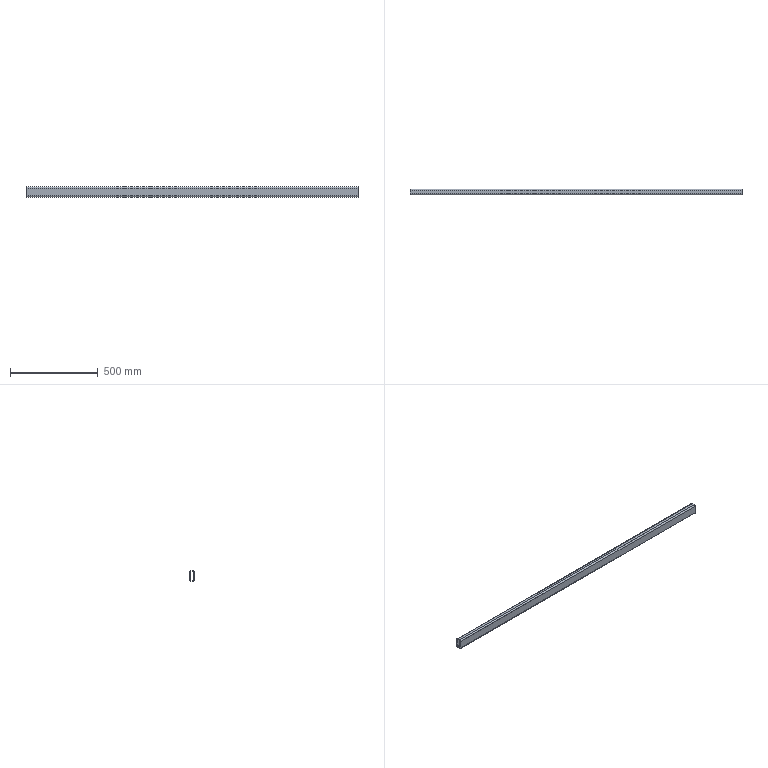Part | STEP file | 1 solid | 18 faces | box 1888 x 30 x 60 mm | volume 1160736 mm3 | plane 10 | cylinder 8 | commonest cylinder face diameters 8 x4 16 x4
STEP:
#1=CARTESIAN_POINT('',(0.,0.,0.));
#2=DIRECTION('',(0.,0.,1.));
#3=DIRECTION('',(1.,0.,0.));
#4=AXIS2_PLACEMENT_3D('',#1,#2,#3);
#5=CARTESIAN_POINT('',(0.,15.,22.));
#6=VERTEX_POINT('',#5);
#7=CARTESIAN_POINT('',(0.,7.,30.));
#8=VERTEX_POINT('',#7);
#9=CARTESIAN_POINT('',(0.,7.,22.));
#10=DIRECTION('',(1.,0.,0.));
#11=DIRECTION('',(0.,0.,-1.));
#12=AXIS2_PLACEMENT_3D('',#9,#10,#11);
#13=CIRCLE('',#12,8.);
#14=CARTESIAN_POINT('',(1888.,7.,22.));
#15=DIRECTION('',(-1.,0.,0.));
#16=DIRECTION('',(0.,0.,1.));
#17=AXIS2_PLACEMENT_3D('',#14,#15,#16);
#18=CYLINDRICAL_SURFACE('',#17,8.);
#19=CARTESIAN_POINT('',(3.142,1888.));
#20=DIRECTION('',(-1.,0.));
#21=VECTOR('',#20,1.);
#22=LINE('',#19,#21);
#23=(GEOMETRIC_REPRESENTATION_CONTEXT(2)PARAMETRIC_REPRESENTATION_CONTEXT()REPRESENTATION_CONTEXT('',''));
#24=DEFINITIONAL_REPRESENTATION('',(#22),#23);
#25=PCURVE('',#18,#24);
#26=CARTESIAN_POINT('',(0.,7.,22.));
#27=DIRECTION('',(1.,0.,0.));
#28=DIRECTION('',(0.,0.,-1.));
#29=AXIS2_PLACEMENT_3D('',#26,#27,#28);
#30=PLANE('',#29);
#31=CARTESIAN_POINT('',(0.,0.));
#32=DIRECTION('',(1.,0.));
#33=AXIS2_PLACEMENT_2D('',#31,#32);
#34=CIRCLE('',#33,8.);
#35=(GEOMETRIC_REPRESENTATION_CONTEXT(2)PARAMETRIC_REPRESENTATION_CONTEXT()REPRESENTATION_CONTEXT('',''));
#36=DEFINITIONAL_REPRESENTATION('',(#34),#35);
#37=PCURVE('',#30,#36);
#38=SURFACE_CURVE('',#13,(#25,#37),.PCURVE_S1.);
#39=EDGE_CURVE('',#6,#8,#38,.T.);
#40=ORIENTED_EDGE('',*,*,#39,.T.);
#41=CARTESIAN_POINT('',(1888.,7.,30.));
#42=VERTEX_POINT('',#41);
#43=CARTESIAN_POINT('',(1888.,7.,30.));
#44=DIRECTION('',(-1.,0.,0.));
#45=VECTOR('',#44,1.);
#46=LINE('',#43,#45);
#47=CARTESIAN_POINT('',(0.,0.));
#48=DIRECTION('',(0.,1.));
#49=VECTOR('',#48,1.);
#50=LINE('',#47,#49);
#51=(GEOMETRIC_REPRESENTATION_CONTEXT(2)PARAMETRIC_REPRESENTATION_CONTEXT()REPRESENTATION_CONTEXT('',''));
#52=DEFINITIONAL_REPRESENTATION('',(#50),#51);
#53=PCURVE('',#18,#52);
#54=CARTESIAN_POINT('',(1888.,7.,30.));
#55=DIRECTION('',(0.,0.,-1.));
#56=DIRECTION('',(-1.,0.,0.));
#57=AXIS2_PLACEMENT_3D('',#54,#55,#56);
#58=PLANE('',#57);
#59=CARTESIAN_POINT('',(0.,0.));
#60=DIRECTION('',(1.,0.));
#61=VECTOR('',#60,1.);
#62=LINE('',#59,#61);
#63=(GEOMETRIC_REPRESENTATION_CONTEXT(2)PARAMETRIC_REPRESENTATION_CONTEXT()REPRESENTATION_CONTEXT('',''));
#64=DEFINITIONAL_REPRESENTATION('',(#62),#63);
#65=PCURVE('',#58,#64);
#66=SURFACE_CURVE('',#46,(#53,#65),.PCURVE_S1.);
#67=EDGE_CURVE('',#42,#8,#66,.T.);
#68=ORIENTED_EDGE('',*,*,#67,.F.);
#69=CARTESIAN_POINT('',(1888.,15.,22.));
#70=VERTEX_POINT('',#69);
#71=CARTESIAN_POINT('',(1888.,7.,22.));
#72=DIRECTION('',(1.,0.,0.));
#73=DIRECTION('',(0.,0.,-1.));
#74=AXIS2_PLACEMENT_3D('',#71,#72,#73);
#75=CIRCLE('',#74,8.);
#76=CARTESIAN_POINT('',(3.142,0.));
#77=DIRECTION('',(-1.,0.));
#78=VECTOR('',#77,1.);
#79=LINE('',#76,#78);
#80=(GEOMETRIC_REPRESENTATION_CONTEXT(2)PARAMETRIC_REPRESENTATION_CONTEXT()REPRESENTATION_CONTEXT('',''));
#81=DEFINITIONAL_REPRESENTATION('',(#79),#80);
#82=PCURVE('',#18,#81);
#83=CARTESIAN_POINT('',(1888.,7.,22.));
#84=DIRECTION('',(1.,0.,0.));
#85=DIRECTION('',(0.,0.,-1.));
#86=AXIS2_PLACEMENT_3D('',#83,#84,#85);
#87=PLANE('',#86);
#88=CARTESIAN_POINT('',(0.,0.));
#89=DIRECTION('',(1.,0.));
#90=AXIS2_PLACEMENT_2D('',#88,#89);
#91=CIRCLE('',#90,8.);
#92=(GEOMETRIC_REPRESENTATION_CONTEXT(2)PARAMETRIC_REPRESENTATION_CONTEXT()REPRESENTATION_CONTEXT('',''));
#93=DEFINITIONAL_REPRESENTATION('',(#91),#92);
#94=PCURVE('',#87,#93);
#95=SURFACE_CURVE('',#75,(#82,#94),.PCURVE_S1.);
#96=EDGE_CURVE('',#70,#42,#95,.T.);
#97=ORIENTED_EDGE('',*,*,#96,.F.);
#98=CARTESIAN_POINT('',(1888.,15.,22.));
#99=DIRECTION('',(-1.,0.,0.));
#100=VECTOR('',#99,1.);
#101=LINE('',#98,#100);
#102=CARTESIAN_POINT('',(1.571,0.));
#103=DIRECTION('',(0.,1.));
#104=VECTOR('',#103,1.);
#105=LINE('',#102,#104);
#106=(GEOMETRIC_REPRESENTATION_CONTEXT(2)PARAMETRIC_REPRESENTATION_CONTEXT()REPRESENTATION_CONTEXT('',''));
#107=DEFINITIONAL_REPRESENTATION('',(#105),#106);
#108=PCURVE('',#18,#107);
#109=CARTESIAN_POINT('',(1888.,15.,22.));
#110=DIRECTION('',(0.,-1.,0.));
#111=DIRECTION('',(0.,0.,-1.));
#112=AXIS2_PLACEMENT_3D('',#109,#110,#111);
#113=PLANE('',#112);
#114=CARTESIAN_POINT('',(0.,0.));
#115=DIRECTION('',(0.,-1.));
#116=VECTOR('',#115,1.);
#117=LINE('',#114,#116);
#118=(GEOMETRIC_REPRESENTATION_CONTEXT(2)PARAMETRIC_REPRESENTATION_CONTEXT()REPRESENTATION_CONTEXT('',''));
#119=DEFINITIONAL_REPRESENTATION('',(#117),#118);
#120=PCURVE('',#113,#119);
#121=SURFACE_CURVE('',#101,(#108,#120),.PCURVE_S1.);
#122=EDGE_CURVE('',#70,#6,#121,.T.);
#123=ORIENTED_EDGE('',*,*,#122,.T.);
#124=EDGE_LOOP('',(#40,#68,#97,#123));
#125=FACE_BOUND('',#124,.T.);
#126=ADVANCED_FACE('',(#125),#18,.T.);
#127=CARTESIAN_POINT('',(0.,-7.,30.));
#128=VERTEX_POINT('',#127);
#129=CARTESIAN_POINT('',(0.,7.,30.));
#130=DIRECTION('',(0.,-1.,0.));
#131=VECTOR('',#130,1.);
#132=LINE('',#129,#131);
#133=CARTESIAN_POINT('',(1888.,0.));
#134=DIRECTION('',(0.,-1.));
#135=VECTOR('',#134,1.);
#136=LINE('',#133,#135);
#137=(GEOMETRIC_REPRESENTATION_CONTEXT(2)PARAMETRIC_REPRESENTATION_CONTEXT()REPRESENTATION_CONTEXT('',''));
#138=DEFINITIONAL_REPRESENTATION('',(#136),#137);
#139=PCURVE('',#58,#138);
#140=CARTESIAN_POINT('',(-8.,0.));
#141=DIRECTION('',(0.,-1.));
#142=VECTOR('',#141,1.);
#143=LINE('',#140,#142);
#144=(GEOMETRIC_REPRESENTATION_CONTEXT(2)PARAMETRIC_REPRESENTATION_CONTEXT()REPRESENTATION_CONTEXT('',''));
#145=DEFINITIONAL_REPRESENTATION('',(#143),#144);
#146=PCURVE('',#30,#145);
#147=SURFACE_CURVE('',#132,(#139,#146),.PCURVE_S1.);
#148=EDGE_CURVE('',#8,#128,#147,.T.);
#149=ORIENTED_EDGE('',*,*,#148,.T.);
#150=CARTESIAN_POINT('',(1888.,-7.,30.));
#151=VERTEX_POINT('',#150);
#152=CARTESIAN_POINT('',(1888.,-7.,30.));
#153=DIRECTION('',(-1.,0.,0.));
#154=VECTOR('',#153,1.);
#155=LINE('',#152,#154);
#156=CARTESIAN_POINT('',(0.,-14.));
#157=DIRECTION('',(1.,0.));
#158=VECTOR('',#157,1.);
#159=LINE('',#156,#158);
#160=(GEOMETRIC_REPRESENTATION_CONTEXT(2)PARAMETRIC_REPRESENTATION_CONTEXT()REPRESENTATION_CONTEXT('',''));
#161=DEFINITIONAL_REPRESENTATION('',(#159),#160);
#162=PCURVE('',#58,#161);
#163=CARTESIAN_POINT('',(1888.,-7.,22.));
#164=DIRECTION('',(-1.,0.,0.));
#165=DIRECTION('',(0.,0.,1.));
#166=AXIS2_PLACEMENT_3D('',#163,#164,#165);
#167=CYLINDRICAL_SURFACE('',#166,8.);
#168=CARTESIAN_POINT('',(6.283,0.));
#169=DIRECTION('',(0.,1.));
#170=VECTOR('',#169,1.);
#171=LINE('',#168,#170);
#172=(GEOMETRIC_REPRESENTATION_CONTEXT(2)PARAMETRIC_REPRESENTATION_CONTEXT()REPRESENTATION_CONTEXT('',''));
#173=DEFINITIONAL_REPRESENTATION('',(#171),#172);
#174=PCURVE('',#167,#173);
#175=SURFACE_CURVE('',#155,(#162,#174),.PCURVE_S1.);
#176=EDGE_CURVE('',#151,#128,#175,.T.);
#177=ORIENTED_EDGE('',*,*,#176,.F.);
#178=CARTESIAN_POINT('',(1888.,7.,30.));
#179=DIRECTION('',(0.,-1.,0.));
#180=VECTOR('',#179,1.);
#181=LINE('',#178,#180);
#182=CARTESIAN_POINT('',(0.,0.));
#183=DIRECTION('',(0.,-1.));
#184=VECTOR('',#183,1.);
#185=LINE('',#182,#184);
#186=(GEOMETRIC_REPRESENTATION_CONTEXT(2)PARAMETRIC_REPRESENTATION_CONTEXT()REPRESENTATION_CONTEXT('',''));
#187=DEFINITIONAL_REPRESENTATION('',(#185),#186);
#188=PCURVE('',#58,#187);
#189=CARTESIAN_POINT('',(-8.,0.));
#190=DIRECTION('',(0.,-1.));
#191=VECTOR('',#190,1.);
#192=LINE('',#189,#191);
#193=(GEOMETRIC_REPRESENTATION_CONTEXT(2)PARAMETRIC_REPRESENTATION_CONTEXT()REPRESENTATION_CONTEXT('',''));
#194=DEFINITIONAL_REPRESENTATION('',(#192),#193);
#195=PCURVE('',#87,#194);
#196=SURFACE_CURVE('',#181,(#188,#195),.PCURVE_S1.);
#197=EDGE_CURVE('',#42,#151,#196,.T.);
#198=ORIENTED_EDGE('',*,*,#197,.F.);
#199=ORIENTED_EDGE('',*,*,#67,.T.);
#200=EDGE_LOOP('',(#149,#177,#198,#199));
#201=FACE_BOUND('',#200,.T.);
#202=ADVANCED_FACE('',(#201),#58,.F.);
#203=CARTESIAN_POINT('',(0.,-15.,22.));
#204=VERTEX_POINT('',#203);
#205=CARTESIAN_POINT('',(0.,-7.,22.));
#206=DIRECTION('',(1.,0.,0.));
#207=DIRECTION('',(0.,0.,-1.));
#208=AXIS2_PLACEMENT_3D('',#205,#206,#207);
#209=CIRCLE('',#208,8.);
#210=CARTESIAN_POINT('',(9.425,1888.));
#211=DIRECTION('',(-1.,0.));
#212=VECTOR('',#211,1.);
#213=LINE('',#210,#212);
#214=(GEOMETRIC_REPRESENTATION_CONTEXT(2)PARAMETRIC_REPRESENTATION_CONTEXT()REPRESENTATION_CONTEXT('',''));
#215=DEFINITIONAL_REPRESENTATION('',(#213),#214);
#216=PCURVE('',#167,#215);
#217=CARTESIAN_POINT('',(0.,-14.));
#218=DIRECTION('',(1.,0.));
#219=AXIS2_PLACEMENT_2D('',#217,#218);
#220=CIRCLE('',#219,8.);
#221=(GEOMETRIC_REPRESENTATION_CONTEXT(2)PARAMETRIC_REPRESENTATION_CONTEXT()REPRESENTATION_CONTEXT('',''));
#222=DEFINITIONAL_REPRESENTATION('',(#220),#221);
#223=PCURVE('',#30,#222);
#224=SURFACE_CURVE('',#209,(#216,#223),.PCURVE_S1.);
#225=EDGE_CURVE('',#128,#204,#224,.T.);
#226=ORIENTED_EDGE('',*,*,#225,.T.);
#227=CARTESIAN_POINT('',(1888.,-15.,22.));
#228=VERTEX_POINT('',#227);
#229=CARTESIAN_POINT('',(1888.,-15.,22.));
#230=DIRECTION('',(-1.,0.,0.));
#231=VECTOR('',#230,1.);
#232=LINE('',#229,#231);
#233=CARTESIAN_POINT('',(4.712,0.));
#234=DIRECTION('',(0.,1.));
#235=VECTOR('',#234,1.);
#236=LINE('',#233,#235);
#237=(GEOMETRIC_REPRESENTATION_CONTEXT(2)PARAMETRIC_REPRESENTATION_CONTEXT()REPRESENTATION_CONTEXT('',''));
#238=DEFINITIONAL_REPRESENTATION('',(#236),#237);
#239=PCURVE('',#167,#238);
#240=CARTESIAN_POINT('',(1888.,-15.,-22.));
#241=DIRECTION('',(0.,1.,0.));
#242=DIRECTION('',(0.,0.,1.));
#243=AXIS2_PLACEMENT_3D('',#240,#241,#242);
#244=PLANE('',#243);
#245=CARTESIAN_POINT('',(44.,0.));
#246=DIRECTION('',(0.,-1.));
#247=VECTOR('',#246,1.);
#248=LINE('',#245,#247);
#249=(GEOMETRIC_REPRESENTATION_CONTEXT(2)PARAMETRIC_REPRESENTATION_CONTEXT()REPRESENTATION_CONTEXT('',''));
#250=DEFINITIONAL_REPRESENTATION('',(#248),#249);
#251=PCURVE('',#244,#250);
#252=SURFACE_CURVE('',#232,(#239,#251),.PCURVE_S1.);
#253=EDGE_CURVE('',#228,#204,#252,.T.);
#254=ORIENTED_EDGE('',*,*,#253,.F.);
#255=CARTESIAN_POINT('',(1888.,-7.,22.));
#256=DIRECTION('',(1.,0.,0.));
#257=DIRECTION('',(0.,0.,-1.));
#258=AXIS2_PLACEMENT_3D('',#255,#256,#257);
#259=CIRCLE('',#258,8.);
#260=CARTESIAN_POINT('',(9.425,0.));
#261=DIRECTION('',(-1.,0.));
#262=VECTOR('',#261,1.);
#263=LINE('',#260,#262);
#264=(GEOMETRIC_REPRESENTATION_CONTEXT(2)PARAMETRIC_REPRESENTATION_CONTEXT()REPRESENTATION_CONTEXT('',''));
#265=DEFINITIONAL_REPRESENTATION('',(#263),#264);
#266=PCURVE('',#167,#265);
#267=CARTESIAN_POINT('',(0.,-14.));
#268=DIRECTION('',(1.,0.));
#269=AXIS2_PLACEMENT_2D('',#267,#268);
#270=CIRCLE('',#269,8.);
#271=(GEOMETRIC_REPRESENTATION_CONTEXT(2)PARAMETRIC_REPRESENTATION_CONTEXT()REPRESENTATION_CONTEXT('',''));
#272=DEFINITIONAL_REPRESENTATION('',(#270),#271);
#273=PCURVE('',#87,#272);
#274=SURFACE_CURVE('',#259,(#266,#273),.PCURVE_S1.);
#275=EDGE_CURVE('',#151,#228,#274,.T.);
#276=ORIENTED_EDGE('',*,*,#275,.F.);
#277=ORIENTED_EDGE('',*,*,#176,.T.);
#278=EDGE_LOOP('',(#226,#254,#276,#277));
#279=FACE_BOUND('',#278,.T.);
#280=ADVANCED_FACE('',(#279),#167,.T.);
#281=CARTESIAN_POINT('',(0.,-15.,-22.));
#282=VERTEX_POINT('',#281);
#283=CARTESIAN_POINT('',(0.,-15.,-22.));
#284=DIRECTION('',(0.,0.,-1.));
#285=VECTOR('',#284,1.);
#286=LINE('',#283,#285);
#287=CARTESIAN_POINT('',(0.,-1888.));
#288=DIRECTION('',(-1.,0.));
#289=VECTOR('',#288,1.);
#290=LINE('',#287,#289);
#291=(GEOMETRIC_REPRESENTATION_CONTEXT(2)PARAMETRIC_REPRESENTATION_CONTEXT()REPRESENTATION_CONTEXT('',''));
#292=DEFINITIONAL_REPRESENTATION('',(#290),#291);
#293=PCURVE('',#244,#292);
#294=CARTESIAN_POINT('',(44.,-22.));
#295=DIRECTION('',(1.,0.));
#296=VECTOR('',#295,1.);
#297=LINE('',#294,#296);
#298=(GEOMETRIC_REPRESENTATION_CONTEXT(2)PARAMETRIC_REPRESENTATION_CONTEXT()REPRESENTATION_CONTEXT('',''));
#299=DEFINITIONAL_REPRESENTATION('',(#297),#298);
#300=PCURVE('',#30,#299);
#301=SURFACE_CURVE('',#286,(#293,#300),.PCURVE_S1.);
#302=EDGE_CURVE('',#204,#282,#301,.T.);
#303=ORIENTED_EDGE('',*,*,#302,.T.);
#304=CARTESIAN_POINT('',(1888.,-15.,-22.));
#305=VERTEX_POINT('',#304);
#306=CARTESIAN_POINT('',(1888.,-15.,-22.));
#307=DIRECTION('',(-1.,0.,0.));
#308=VECTOR('',#307,1.);
#309=LINE('',#306,#308);
#310=CARTESIAN_POINT('',(0.,0.));
#311=DIRECTION('',(0.,-1.));
#312=VECTOR('',#311,1.);
#313=LINE('',#310,#312);
#314=(GEOMETRIC_REPRESENTATION_CONTEXT(2)PARAMETRIC_REPRESENTATION_CONTEXT()REPRESENTATION_CONTEXT('',''));
#315=DEFINITIONAL_REPRESENTATION('',(#313),#314);
#316=PCURVE('',#244,#315);
#317=CARTESIAN_POINT('',(1888.,-7.,-22.));
#318=DIRECTION('',(-1.,0.,0.));
#319=DIRECTION('',(0.,0.,1.));
#320=AXIS2_PLACEMENT_3D('',#317,#318,#319);
#321=CYLINDRICAL_SURFACE('',#320,8.);
#322=CARTESIAN_POINT('',(4.712,0.));
#323=DIRECTION('',(0.,1.));
#324=VECTOR('',#323,1.);
#325=LINE('',#322,#324);
#326=(GEOMETRIC_REPRESENTATION_CONTEXT(2)PARAMETRIC_REPRESENTATION_CONTEXT()REPRESENTATION_CONTEXT('',''));
#327=DEFINITIONAL_REPRESENTATION('',(#325),#326);
#328=PCURVE('',#321,#327);
#329=SURFACE_CURVE('',#309,(#316,#328),.PCURVE_S1.);
#330=EDGE_CURVE('',#305,#282,#329,.T.);
#331=ORIENTED_EDGE('',*,*,#330,.F.);
#332=CARTESIAN_POINT('',(1888.,-15.,-22.));
#333=DIRECTION('',(0.,0.,-1.));
#334=VECTOR('',#333,1.);
#335=LINE('',#332,#334);
#336=CARTESIAN_POINT('',(0.,0.));
#337=DIRECTION('',(-1.,0.));
#338=VECTOR('',#337,1.);
#339=LINE('',#336,#338);
#340=(GEOMETRIC_REPRESENTATION_CONTEXT(2)PARAMETRIC_REPRESENTATION_CONTEXT()REPRESENTATION_CONTEXT('',''));
#341=DEFINITIONAL_REPRESENTATION('',(#339),#340);
#342=PCURVE('',#244,#341);
#343=CARTESIAN_POINT('',(44.,-22.));
#344=DIRECTION('',(1.,0.));
#345=VECTOR('',#344,1.);
#346=LINE('',#343,#345);
#347=(GEOMETRIC_REPRESENTATION_CONTEXT(2)PARAMETRIC_REPRESENTATION_CONTEXT()REPRESENTATION_CONTEXT('',''));
#348=DEFINITIONAL_REPRESENTATION('',(#346),#347);
#349=PCURVE('',#87,#348);
#350=SURFACE_CURVE('',#335,(#342,#349),.PCURVE_S1.);
#351=EDGE_CURVE('',#228,#305,#350,.T.);
#352=ORIENTED_EDGE('',*,*,#351,.F.);
#353=ORIENTED_EDGE('',*,*,#253,.T.);
#354=EDGE_LOOP('',(#303,#331,#352,#353));
#355=FACE_BOUND('',#354,.T.);
#356=ADVANCED_FACE('',(#355),#244,.F.);
#357=CARTESIAN_POINT('',(0.,-7.,-30.));
#358=VERTEX_POINT('',#357);
#359=CARTESIAN_POINT('',(0.,-7.,-22.));
#360=DIRECTION('',(1.,0.,0.));
#361=DIRECTION('',(0.,0.,-1.));
#362=AXIS2_PLACEMENT_3D('',#359,#360,#361);
#363=CIRCLE('',#362,8.);
#364=CARTESIAN_POINT('',(9.425,1888.));
#365=DIRECTION('',(-1.,0.));
#366=VECTOR('',#365,1.);
#367=LINE('',#364,#366);
#368=(GEOMETRIC_REPRESENTATION_CONTEXT(2)PARAMETRIC_REPRESENTATION_CONTEXT()REPRESENTATION_CONTEXT('',''));
#369=DEFINITIONAL_REPRESENTATION('',(#367),#368);
#370=PCURVE('',#321,#369);
#371=CARTESIAN_POINT('',(44.,-14.));
#372=DIRECTION('',(1.,0.));
#373=AXIS2_PLACEMENT_2D('',#371,#372);
#374=CIRCLE('',#373,8.);
#375=(GEOMETRIC_REPRESENTATION_CONTEXT(2)PARAMETRIC_REPRESENTATION_CONTEXT()REPRESENTATION_CONTEXT('',''));
#376=DEFINITIONAL_REPRESENTATION('',(#374),#375);
#377=PCURVE('',#30,#376);
#378=SURFACE_CURVE('',#363,(#370,#377),.PCURVE_S1.);
#379=EDGE_CURVE('',#282,#358,#378,.T.);
#380=ORIENTED_EDGE('',*,*,#379,.T.);
#381=CARTESIAN_POINT('',(1888.,-7.,-30.));
#382=VERTEX_POINT('',#381);
#383=CARTESIAN_POINT('',(1888.,-7.,-30.));
#384=DIRECTION('',(-1.,0.,0.));
#385=VECTOR('',#384,1.);
#386=LINE('',#383,#385);
#387=CARTESIAN_POINT('',(3.142,0.));
#388=DIRECTION('',(0.,1.));
#389=VECTOR('',#388,1.);
#390=LINE('',#387,#389);
#391=(GEOMETRIC_REPRESENTATION_CONTEXT(2)PARAMETRIC_REPRESENTATION_CONTEXT()REPRESENTATION_CONTEXT('',''));
#392=DEFINITIONAL_REPRESENTATION('',(#390),#391);
#393=PCURVE('',#321,#392);
#394=CARTESIAN_POINT('',(1888.,-7.,-30.));
#395=DIRECTION('',(0.,0.,1.));
#396=DIRECTION('',(1.,0.,0.));
#397=AXIS2_PLACEMENT_3D('',#394,#395,#396);
#398=PLANE('',#397);
#399=CARTESIAN_POINT('',(0.,0.));
#400=DIRECTION('',(-1.,0.));
#401=VECTOR('',#400,1.);
#402=LINE('',#399,#401);
#403=(GEOMETRIC_REPRESENTATION_CONTEXT(2)PARAMETRIC_REPRESENTATION_CONTEXT()REPRESENTATION_CONTEXT('',''));
#404=DEFINITIONAL_REPRESENTATION('',(#402),#403);
#405=PCURVE('',#398,#404);
#406=SURFACE_CURVE('',#386,(#393,#405),.PCURVE_S1.);
#407=EDGE_CURVE('',#382,#358,#406,.T.);
#408=ORIENTED_EDGE('',*,*,#407,.F.);
#409=CARTESIAN_POINT('',(1888.,-7.,-22.));
#410=DIRECTION('',(1.,0.,0.));
#411=DIRECTION('',(0.,0.,-1.));
#412=AXIS2_PLACEMENT_3D('',#409,#410,#411);
#413=CIRCLE('',#412,8.);
#414=CARTESIAN_POINT('',(9.425,0.));
#415=DIRECTION('',(-1.,0.));
#416=VECTOR('',#415,1.);
#417=LINE('',#414,#416);
#418=(GEOMETRIC_REPRESENTATION_CONTEXT(2)PARAMETRIC_REPRESENTATION_CONTEXT()REPRESENTATION_CONTEXT('',''));
#419=DEFINITIONAL_REPRESENTATION('',(#417),#418);
#420=PCURVE('',#321,#419);
#421=CARTESIAN_POINT('',(44.,-14.));
#422=DIRECTION('',(1.,0.));
#423=AXIS2_PLACEMENT_2D('',#421,#422);
#424=CIRCLE('',#423,8.);
#425=(GEOMETRIC_REPRESENTATION_CONTEXT(2)PARAMETRIC_REPRESENTATION_CONTEXT()REPRESENTATION_CONTEXT('',''));
#426=DEFINITIONAL_REPRESENTATION('',(#424),#425);
#427=PCURVE('',#87,#426);
#428=SURFACE_CURVE('',#413,(#420,#427),.PCURVE_S1.);
#429=EDGE_CURVE('',#305,#382,#428,.T.);
#430=ORIENTED_EDGE('',*,*,#429,.F.);
#431=ORIENTED_EDGE('',*,*,#330,.T.);
#432=EDGE_LOOP('',(#380,#408,#430,#431));
#433=FACE_BOUND('',#432,.T.);
#434=ADVANCED_FACE('',(#433),#321,.T.);
#435=CARTESIAN_POINT('',(0.,7.,-30.));
#436=VERTEX_POINT('',#435);
#437=CARTESIAN_POINT('',(0.,-7.,-30.));
#438=DIRECTION('',(0.,1.,0.));
#439=VECTOR('',#438,1.);
#440=LINE('',#437,#439);
#441=CARTESIAN_POINT('',(-1888.,0.));
#442=DIRECTION('',(0.,1.));
#443=VECTOR('',#442,1.);
#444=LINE('',#441,#443);
#445=(GEOMETRIC_REPRESENTATION_CONTEXT(2)PARAMETRIC_REPRESENTATION_CONTEXT()REPRESENTATION_CONTEXT('',''));
#446=DEFINITIONAL_REPRESENTATION('',(#444),#445);
#447=PCURVE('',#398,#446);
#448=CARTESIAN_POINT('',(52.,-14.));
#449=DIRECTION('',(0.,1.));
#450=VECTOR('',#449,1.);
#451=LINE('',#448,#450);
#452=(GEOMETRIC_REPRESENTATION_CONTEXT(2)PARAMETRIC_REPRESENTATION_CONTEXT()REPRESENTATION_CONTEXT('',''));
#453=DEFINITIONAL_REPRESENTATION('',(#451),#452);
#454=PCURVE('',#30,#453);
#455=SURFACE_CURVE('',#440,(#447,#454),.PCURVE_S1.);
#456=EDGE_CURVE('',#358,#436,#455,.T.);
#457=ORIENTED_EDGE('',*,*,#456,.T.);
#458=CARTESIAN_POINT('',(1888.,7.,-30.));
#459=VERTEX_POINT('',#458);
#460=CARTESIAN_POINT('',(1888.,7.,-30.));
#461=DIRECTION('',(-1.,0.,0.));
#462=VECTOR('',#461,1.);
#463=LINE('',#460,#462);
#464=CARTESIAN_POINT('',(0.,14.));
#465=DIRECTION('',(-1.,0.));
#466=VECTOR('',#465,1.);
#467=LINE('',#464,#466);
#468=(GEOMETRIC_REPRESENTATION_CONTEXT(2)PARAMETRIC_REPRESENTATION_CONTEXT()REPRESENTATION_CONTEXT('',''));
#469=DEFINITIONAL_REPRESENTATION('',(#467),#468);
#470=PCURVE('',#398,#469);
#471=CARTESIAN_POINT('',(1888.,7.,-22.));
#472=DIRECTION('',(-1.,0.,0.));
#473=DIRECTION('',(0.,0.,1.));
#474=AXIS2_PLACEMENT_3D('',#471,#472,#473);
#475=CYLINDRICAL_SURFACE('',#474,8.);
#476=CARTESIAN_POINT('',(3.142,0.));
#477=DIRECTION('',(0.,1.));
#478=VECTOR('',#477,1.);
#479=LINE('',#476,#478);
#480=(GEOMETRIC_REPRESENTATION_CONTEXT(2)PARAMETRIC_REPRESENTATION_CONTEXT()REPRESENTATION_CONTEXT('',''));
#481=DEFINITIONAL_REPRESENTATION('',(#479),#480);
#482=PCURVE('',#475,#481);
#483=SURFACE_CURVE('',#463,(#470,#482),.PCURVE_S1.);
#484=EDGE_CURVE('',#459,#436,#483,.T.);
#485=ORIENTED_EDGE('',*,*,#484,.F.);
#486=CARTESIAN_POINT('',(1888.,-7.,-30.));
#487=DIRECTION('',(0.,1.,0.));
#488=VECTOR('',#487,1.);
#489=LINE('',#486,#488);
#490=CARTESIAN_POINT('',(0.,0.));
#491=DIRECTION('',(0.,1.));
#492=VECTOR('',#491,1.);
#493=LINE('',#490,#492);
#494=(GEOMETRIC_REPRESENTATION_CONTEXT(2)PARAMETRIC_REPRESENTATION_CONTEXT()REPRESENTATION_CONTEXT('',''));
#495=DEFINITIONAL_REPRESENTATION('',(#493),#494);
#496=PCURVE('',#398,#495);
#497=CARTESIAN_POINT('',(52.,-14.));
#498=DIRECTION('',(0.,1.));
#499=VECTOR('',#498,1.);
#500=LINE('',#497,#499);
#501=(GEOMETRIC_REPRESENTATION_CONTEXT(2)PARAMETRIC_REPRESENTATION_CONTEXT()REPRESENTATION_CONTEXT('',''));
#502=DEFINITIONAL_REPRESENTATION('',(#500),#501);
#503=PCURVE('',#87,#502);
#504=SURFACE_CURVE('',#489,(#496,#503),.PCURVE_S1.);
#505=EDGE_CURVE('',#382,#459,#504,.T.);
#506=ORIENTED_EDGE('',*,*,#505,.F.);
#507=ORIENTED_EDGE('',*,*,#407,.T.);
#508=EDGE_LOOP('',(#457,#485,#506,#507));
#509=FACE_BOUND('',#508,.T.);
#510=ADVANCED_FACE('',(#509),#398,.F.);
#511=CARTESIAN_POINT('',(0.,15.,-22.));
#512=VERTEX_POINT('',#511);
#513=CARTESIAN_POINT('',(0.,7.,-22.));
#514=DIRECTION('',(1.,0.,0.));
#515=DIRECTION('',(0.,0.,-1.));
#516=AXIS2_PLACEMENT_3D('',#513,#514,#515);
#517=CIRCLE('',#516,8.);
#518=CARTESIAN_POINT('',(3.142,1888.));
#519=DIRECTION('',(-1.,0.));
#520=VECTOR('',#519,1.);
#521=LINE('',#518,#520);
#522=(GEOMETRIC_REPRESENTATION_CONTEXT(2)PARAMETRIC_REPRESENTATION_CONTEXT()REPRESENTATION_CONTEXT('',''));
#523=DEFINITIONAL_REPRESENTATION('',(#521),#522);
#524=PCURVE('',#475,#523);
#525=CARTESIAN_POINT('',(44.,0.));
#526=DIRECTION('',(1.,0.));
#527=AXIS2_PLACEMENT_2D('',#525,#526);
#528=CIRCLE('',#527,8.);
#529=(GEOMETRIC_REPRESENTATION_CONTEXT(2)PARAMETRIC_REPRESENTATION_CONTEXT()REPRESENTATION_CONTEXT('',''));
#530=DEFINITIONAL_REPRESENTATION('',(#528),#529);
#531=PCURVE('',#30,#530);
#532=SURFACE_CURVE('',#517,(#524,#531),.PCURVE_S1.);
#533=EDGE_CURVE('',#436,#512,#532,.T.);
#534=ORIENTED_EDGE('',*,*,#533,.T.);
#535=CARTESIAN_POINT('',(1888.,15.,-22.));
#536=VERTEX_POINT('',#535);
#537=CARTESIAN_POINT('',(1888.,15.,-22.));
#538=DIRECTION('',(-1.,0.,0.));
#539=VECTOR('',#538,1.);
#540=LINE('',#537,#539);
#541=CARTESIAN_POINT('',(1.571,0.));
#542=DIRECTION('',(0.,1.));
#543=VECTOR('',#542,1.);
#544=LINE('',#541,#543);
#545=(GEOMETRIC_REPRESENTATION_CONTEXT(2)PARAMETRIC_REPRESENTATION_CONTEXT()REPRESENTATION_CONTEXT('',''));
#546=DEFINITIONAL_REPRESENTATION('',(#544),#545);
#547=PCURVE('',#475,#546);
#548=CARTESIAN_POINT('',(44.,0.));
#549=DIRECTION('',(0.,-1.));
#550=VECTOR('',#549,1.);
#551=LINE('',#548,#550);
#552=(GEOMETRIC_REPRESENTATION_CONTEXT(2)PARAMETRIC_REPRESENTATION_CONTEXT()REPRESENTATION_CONTEXT('',''));
#553=DEFINITIONAL_REPRESENTATION('',(#551),#552);
#554=PCURVE('',#113,#553);
#555=SURFACE_CURVE('',#540,(#547,#554),.PCURVE_S1.);
#556=EDGE_CURVE('',#536,#512,#555,.T.);
#557=ORIENTED_EDGE('',*,*,#556,.F.);
#558=CARTESIAN_POINT('',(1888.,7.,-22.));
#559=DIRECTION('',(1.,0.,0.));
#560=DIRECTION('',(0.,0.,-1.));
#561=AXIS2_PLACEMENT_3D('',#558,#559,#560);
#562=CIRCLE('',#561,8.);
#563=CARTESIAN_POINT('',(3.142,0.));
#564=DIRECTION('',(-1.,0.));
#565=VECTOR('',#564,1.);
#566=LINE('',#563,#565);
#567=(GEOMETRIC_REPRESENTATION_CONTEXT(2)PARAMETRIC_REPRESENTATION_CONTEXT()REPRESENTATION_CONTEXT('',''));
#568=DEFINITIONAL_REPRESENTATION('',(#566),#567);
#569=PCURVE('',#475,#568);
#570=CARTESIAN_POINT('',(44.,0.));
#571=DIRECTION('',(1.,0.));
#572=AXIS2_PLACEMENT_2D('',#570,#571);
#573=CIRCLE('',#572,8.);
#574=(GEOMETRIC_REPRESENTATION_CONTEXT(2)PARAMETRIC_REPRESENTATION_CONTEXT()REPRESENTATION_CONTEXT('',''));
#575=DEFINITIONAL_REPRESENTATION('',(#573),#574);
#576=PCURVE('',#87,#575);
#577=SURFACE_CURVE('',#562,(#569,#576),.PCURVE_S1.);
#578=EDGE_CURVE('',#459,#536,#577,.T.);
#579=ORIENTED_EDGE('',*,*,#578,.F.);
#580=ORIENTED_EDGE('',*,*,#484,.T.);
#581=EDGE_LOOP('',(#534,#557,#579,#580));
#582=FACE_BOUND('',#581,.T.);
#583=ADVANCED_FACE('',(#582),#475,.T.);
#584=CARTESIAN_POINT('',(1888.,-11.,22.));
#585=VERTEX_POINT('',#584);
#586=CARTESIAN_POINT('',(0.,-11.,22.));
#587=VERTEX_POINT('',#586);
#588=CARTESIAN_POINT('',(1888.,-11.,22.));
#589=DIRECTION('',(-1.,0.,0.));
#590=VECTOR('',#589,1.);
#591=LINE('',#588,#590);
#592=CARTESIAN_POINT('',(1888.,-7.,22.));
#593=DIRECTION('',(-1.,0.,0.));
#594=DIRECTION('',(0.,0.,1.));
#595=AXIS2_PLACEMENT_3D('',#592,#593,#594);
#596=CYLINDRICAL_SURFACE('',#595,4.);
#597=CARTESIAN_POINT('',(4.712,0.));
#598=DIRECTION('',(0.,1.));
#599=VECTOR('',#598,1.);
#600=LINE('',#597,#599);
#601=(GEOMETRIC_REPRESENTATION_CONTEXT(2)PARAMETRIC_REPRESENTATION_CONTEXT()REPRESENTATION_CONTEXT('',''));
#602=DEFINITIONAL_REPRESENTATION('',(#600),#601);
#603=PCURVE('',#596,#602);
#604=CARTESIAN_POINT('',(1888.,-11.,-22.));
#605=DIRECTION('',(0.,1.,0.));
#606=DIRECTION('',(0.,0.,1.));
#607=AXIS2_PLACEMENT_3D('',#604,#605,#606);
#608=PLANE('',#607);
#609=CARTESIAN_POINT('',(44.,0.));
#610=DIRECTION('',(0.,-1.));
#611=VECTOR('',#610,1.);
#612=LINE('',#609,#611);
#613=(GEOMETRIC_REPRESENTATION_CONTEXT(2)PARAMETRIC_REPRESENTATION_CONTEXT()REPRESENTATION_CONTEXT('',''));
#614=DEFINITIONAL_REPRESENTATION('',(#612),#613);
#615=PCURVE('',#608,#614);
#616=SURFACE_CURVE('',#591,(#603,#615),.PCURVE_S1.);
#617=EDGE_CURVE('',#585,#587,#616,.T.);
#618=ORIENTED_EDGE('',*,*,#617,.F.);
#619=CARTESIAN_POINT('',(1888.,-7.,26.));
#620=VERTEX_POINT('',#619);
#621=CARTESIAN_POINT('',(1888.,-7.,22.));
#622=DIRECTION('',(1.,0.,0.));
#623=DIRECTION('',(0.,0.,-1.));
#624=AXIS2_PLACEMENT_3D('',#621,#622,#623);
#625=CIRCLE('',#624,4.);
#626=CARTESIAN_POINT('',(9.425,0.));
#627=DIRECTION('',(-1.,0.));
#628=VECTOR('',#627,1.);
#629=LINE('',#626,#628);
#630=(GEOMETRIC_REPRESENTATION_CONTEXT(2)PARAMETRIC_REPRESENTATION_CONTEXT()REPRESENTATION_CONTEXT('',''));
#631=DEFINITIONAL_REPRESENTATION('',(#629),#630);
#632=PCURVE('',#596,#631);
#633=CARTESIAN_POINT('',(0.,-14.));
#634=DIRECTION('',(1.,0.));
#635=AXIS2_PLACEMENT_2D('',#633,#634);
#636=CIRCLE('',#635,4.);
#637=(GEOMETRIC_REPRESENTATION_CONTEXT(2)PARAMETRIC_REPRESENTATION_CONTEXT()REPRESENTATION_CONTEXT('',''));
#638=DEFINITIONAL_REPRESENTATION('',(#636),#637);
#639=PCURVE('',#87,#638);
#640=SURFACE_CURVE('',#625,(#632,#639),.PCURVE_S1.);
#641=EDGE_CURVE('',#620,#585,#640,.T.);
#642=ORIENTED_EDGE('',*,*,#641,.F.);
#643=CARTESIAN_POINT('',(0.,-7.,26.));
#644=VERTEX_POINT('',#643);
#645=CARTESIAN_POINT('',(1888.,-7.,26.));
#646=DIRECTION('',(-1.,0.,0.));
#647=VECTOR('',#646,1.);
#648=LINE('',#645,#647);
#649=CARTESIAN_POINT('',(6.283,0.));
#650=DIRECTION('',(0.,1.));
#651=VECTOR('',#650,1.);
#652=LINE('',#649,#651);
#653=(GEOMETRIC_REPRESENTATION_CONTEXT(2)PARAMETRIC_REPRESENTATION_CONTEXT()REPRESENTATION_CONTEXT('',''));
#654=DEFINITIONAL_REPRESENTATION('',(#652),#653);
#655=PCURVE('',#596,#654);
#656=CARTESIAN_POINT('',(1888.,7.,26.));
#657=DIRECTION('',(0.,0.,-1.));
#658=DIRECTION('',(-1.,0.,0.));
#659=AXIS2_PLACEMENT_3D('',#656,#657,#658);
#660=PLANE('',#659);
#661=CARTESIAN_POINT('',(0.,-14.));
#662=DIRECTION('',(1.,0.));
#663=VECTOR('',#662,1.);
#664=LINE('',#661,#663);
#665=(GEOMETRIC_REPRESENTATION_CONTEXT(2)PARAMETRIC_REPRESENTATION_CONTEXT()REPRESENTATION_CONTEXT('',''));
#666=DEFINITIONAL_REPRESENTATION('',(#664),#665);
#667=PCURVE('',#660,#666);
#668=SURFACE_CURVE('',#648,(#655,#667),.PCURVE_S1.);
#669=EDGE_CURVE('',#620,#644,#668,.T.);
#670=ORIENTED_EDGE('',*,*,#669,.T.);
#671=CARTESIAN_POINT('',(0.,-7.,22.));
#672=DIRECTION('',(1.,0.,0.));
#673=DIRECTION('',(0.,0.,-1.));
#674=AXIS2_PLACEMENT_3D('',#671,#672,#673);
#675=CIRCLE('',#674,4.);
#676=CARTESIAN_POINT('',(9.425,1888.));
#677=DIRECTION('',(-1.,0.));
#678=VECTOR('',#677,1.);
#679=LINE('',#676,#678);
#680=(GEOMETRIC_REPRESENTATION_CONTEXT(2)PARAMETRIC_REPRESENTATION_CONTEXT()REPRESENTATION_CONTEXT('',''));
#681=DEFINITIONAL_REPRESENTATION('',(#679),#680);
#682=PCURVE('',#596,#681);
#683=CARTESIAN_POINT('',(0.,-14.));
#684=DIRECTION('',(1.,0.));
#685=AXIS2_PLACEMENT_2D('',#683,#684);
#686=CIRCLE('',#685,4.);
#687=(GEOMETRIC_REPRESENTATION_CONTEXT(2)PARAMETRIC_REPRESENTATION_CONTEXT()REPRESENTATION_CONTEXT('',''));
#688=DEFINITIONAL_REPRESENTATION('',(#686),#687);
#689=PCURVE('',#30,#688);
#690=SURFACE_CURVE('',#675,(#682,#689),.PCURVE_S1.);
#691=EDGE_CURVE('',#644,#587,#690,.T.);
#692=ORIENTED_EDGE('',*,*,#691,.T.);
#693=EDGE_LOOP('',(#618,#642,#670,#692));
#694=FACE_BOUND('',#693,.F.);
#695=ADVANCED_FACE('',(#694),#596,.F.);
#696=CARTESIAN_POINT('',(0.,7.,26.));
#697=VERTEX_POINT('',#696);
#698=CARTESIAN_POINT('',(0.,7.,26.));
#699=DIRECTION('',(0.,-1.,0.));
#700=VECTOR('',#699,1.);
#701=LINE('',#698,#700);
#702=CARTESIAN_POINT('',(1888.,0.));
#703=DIRECTION('',(0.,-1.));
#704=VECTOR('',#703,1.);
#705=LINE('',#702,#704);
#706=(GEOMETRIC_REPRESENTATION_CONTEXT(2)PARAMETRIC_REPRESENTATION_CONTEXT()REPRESENTATION_CONTEXT('',''));
#707=DEFINITIONAL_REPRESENTATION('',(#705),#706);
#708=PCURVE('',#660,#707);
#709=CARTESIAN_POINT('',(-4.,0.));
#710=DIRECTION('',(0.,-1.));
#711=VECTOR('',#710,1.);
#712=LINE('',#709,#711);
#713=(GEOMETRIC_REPRESENTATION_CONTEXT(2)PARAMETRIC_REPRESENTATION_CONTEXT()REPRESENTATION_CONTEXT('',''));
#714=DEFINITIONAL_REPRESENTATION('',(#712),#713);
#715=PCURVE('',#30,#714);
#716=SURFACE_CURVE('',#701,(#708,#715),.PCURVE_S1.);
#717=EDGE_CURVE('',#697,#644,#716,.T.);
#718=ORIENTED_EDGE('',*,*,#717,.F.);
#719=CARTESIAN_POINT('',(1888.,7.,26.));
#720=VERTEX_POINT('',#719);
#721=CARTESIAN_POINT('',(1888.,7.,26.));
#722=DIRECTION('',(-1.,0.,0.));
#723=VECTOR('',#722,1.);
#724=LINE('',#721,#723);
#725=CARTESIAN_POINT('',(0.,0.));
#726=DIRECTION('',(1.,0.));
#727=VECTOR('',#726,1.);
#728=LINE('',#725,#727);
#729=(GEOMETRIC_REPRESENTATION_CONTEXT(2)PARAMETRIC_REPRESENTATION_CONTEXT()REPRESENTATION_CONTEXT('',''));
#730=DEFINITIONAL_REPRESENTATION('',(#728),#729);
#731=PCURVE('',#660,#730);
#732=CARTESIAN_POINT('',(1888.,7.,22.));
#733=DIRECTION('',(-1.,0.,0.));
#734=DIRECTION('',(0.,0.,1.));
#735=AXIS2_PLACEMENT_3D('',#732,#733,#734);
#736=CYLINDRICAL_SURFACE('',#735,4.);
#737=CARTESIAN_POINT('',(0.,0.));
#738=DIRECTION('',(0.,1.));
#739=VECTOR('',#738,1.);
#740=LINE('',#737,#739);
#741=(GEOMETRIC_REPRESENTATION_CONTEXT(2)PARAMETRIC_REPRESENTATION_CONTEXT()REPRESENTATION_CONTEXT('',''));
#742=DEFINITIONAL_REPRESENTATION('',(#740),#741);
#743=PCURVE('',#736,#742);
#744=SURFACE_CURVE('',#724,(#731,#743),.PCURVE_S1.);
#745=EDGE_CURVE('',#720,#697,#744,.T.);
#746=ORIENTED_EDGE('',*,*,#745,.F.);
#747=CARTESIAN_POINT('',(1888.,7.,26.));
#748=DIRECTION('',(0.,-1.,0.));
#749=VECTOR('',#748,1.);
#750=LINE('',#747,#749);
#751=CARTESIAN_POINT('',(0.,0.));
#752=DIRECTION('',(0.,-1.));
#753=VECTOR('',#752,1.);
#754=LINE('',#751,#753);
#755=(GEOMETRIC_REPRESENTATION_CONTEXT(2)PARAMETRIC_REPRESENTATION_CONTEXT()REPRESENTATION_CONTEXT('',''));
#756=DEFINITIONAL_REPRESENTATION('',(#754),#755);
#757=PCURVE('',#660,#756);
#758=CARTESIAN_POINT('',(-4.,0.));
#759=DIRECTION('',(0.,-1.));
#760=VECTOR('',#759,1.);
#761=LINE('',#758,#760);
#762=(GEOMETRIC_REPRESENTATION_CONTEXT(2)PARAMETRIC_REPRESENTATION_CONTEXT()REPRESENTATION_CONTEXT('',''));
#763=DEFINITIONAL_REPRESENTATION('',(#761),#762);
#764=PCURVE('',#87,#763);
#765=SURFACE_CURVE('',#750,(#757,#764),.PCURVE_S1.);
#766=EDGE_CURVE('',#720,#620,#765,.T.);
#767=ORIENTED_EDGE('',*,*,#766,.T.);
#768=ORIENTED_EDGE('',*,*,#669,.T.);
#769=EDGE_LOOP('',(#718,#746,#767,#768));
#770=FACE_BOUND('',#769,.T.);
#771=ADVANCED_FACE('',(#770),#660,.T.);
#772=ORIENTED_EDGE('',*,*,#745,.F.);
#773=CARTESIAN_POINT('',(1888.,11.,22.));
#774=VERTEX_POINT('',#773);
#775=CARTESIAN_POINT('',(1888.,7.,22.));
#776=DIRECTION('',(1.,0.,0.));
#777=DIRECTION('',(0.,0.,-1.));
#778=AXIS2_PLACEMENT_3D('',#775,#776,#777);
#779=CIRCLE('',#778,4.);
#780=CARTESIAN_POINT('',(3.142,0.));
#781=DIRECTION('',(-1.,0.));
#782=VECTOR('',#781,1.);
#783=LINE('',#780,#782);
#784=(GEOMETRIC_REPRESENTATION_CONTEXT(2)PARAMETRIC_REPRESENTATION_CONTEXT()REPRESENTATION_CONTEXT('',''));
#785=DEFINITIONAL_REPRESENTATION('',(#783),#784);
#786=PCURVE('',#736,#785);
#787=CARTESIAN_POINT('',(0.,0.));
#788=DIRECTION('',(1.,0.));
#789=AXIS2_PLACEMENT_2D('',#787,#788);
#790=CIRCLE('',#789,4.);
#791=(GEOMETRIC_REPRESENTATION_CONTEXT(2)PARAMETRIC_REPRESENTATION_CONTEXT()REPRESENTATION_CONTEXT('',''));
#792=DEFINITIONAL_REPRESENTATION('',(#790),#791);
#793=PCURVE('',#87,#792);
#794=SURFACE_CURVE('',#779,(#786,#793),.PCURVE_S1.);
#795=EDGE_CURVE('',#774,#720,#794,.T.);
#796=ORIENTED_EDGE('',*,*,#795,.F.);
#797=CARTESIAN_POINT('',(0.,11.,22.));
#798=VERTEX_POINT('',#797);
#799=CARTESIAN_POINT('',(1888.,11.,22.));
#800=DIRECTION('',(-1.,0.,0.));
#801=VECTOR('',#800,1.);
#802=LINE('',#799,#801);
#803=CARTESIAN_POINT('',(1.571,0.));
#804=DIRECTION('',(0.,1.));
#805=VECTOR('',#804,1.);
#806=LINE('',#803,#805);
#807=(GEOMETRIC_REPRESENTATION_CONTEXT(2)PARAMETRIC_REPRESENTATION_CONTEXT()REPRESENTATION_CONTEXT('',''));
#808=DEFINITIONAL_REPRESENTATION('',(#806),#807);
#809=PCURVE('',#736,#808);
#810=CARTESIAN_POINT('',(1888.,11.,22.));
#811=DIRECTION('',(0.,-1.,0.));
#812=DIRECTION('',(0.,0.,-1.));
#813=AXIS2_PLACEMENT_3D('',#810,#811,#812);
#814=PLANE('',#813);
#815=CARTESIAN_POINT('',(0.,0.));
#816=DIRECTION('',(0.,-1.));
#817=VECTOR('',#816,1.);
#818=LINE('',#815,#817);
#819=(GEOMETRIC_REPRESENTATION_CONTEXT(2)PARAMETRIC_REPRESENTATION_CONTEXT()REPRESENTATION_CONTEXT('',''));
#820=DEFINITIONAL_REPRESENTATION('',(#818),#819);
#821=PCURVE('',#814,#820);
#822=SURFACE_CURVE('',#802,(#809,#821),.PCURVE_S1.);
#823=EDGE_CURVE('',#774,#798,#822,.T.);
#824=ORIENTED_EDGE('',*,*,#823,.T.);
#825=CARTESIAN_POINT('',(0.,7.,22.));
#826=DIRECTION('',(1.,0.,0.));
#827=DIRECTION('',(0.,0.,-1.));
#828=AXIS2_PLACEMENT_3D('',#825,#826,#827);
#829=CIRCLE('',#828,4.);
#830=CARTESIAN_POINT('',(3.142,1888.));
#831=DIRECTION('',(-1.,0.));
#832=VECTOR('',#831,1.);
#833=LINE('',#830,#832);
#834=(GEOMETRIC_REPRESENTATION_CONTEXT(2)PARAMETRIC_REPRESENTATION_CONTEXT()REPRESENTATION_CONTEXT('',''));
#835=DEFINITIONAL_REPRESENTATION('',(#833),#834);
#836=PCURVE('',#736,#835);
#837=CARTESIAN_POINT('',(0.,0.));
#838=DIRECTION('',(1.,0.));
#839=AXIS2_PLACEMENT_2D('',#837,#838);
#840=CIRCLE('',#839,4.);
#841=(GEOMETRIC_REPRESENTATION_CONTEXT(2)PARAMETRIC_REPRESENTATION_CONTEXT()REPRESENTATION_CONTEXT('',''));
#842=DEFINITIONAL_REPRESENTATION('',(#840),#841);
#843=PCURVE('',#30,#842);
#844=SURFACE_CURVE('',#829,(#836,#843),.PCURVE_S1.);
#845=EDGE_CURVE('',#798,#697,#844,.T.);
#846=ORIENTED_EDGE('',*,*,#845,.T.);
#847=EDGE_LOOP('',(#772,#796,#824,#846));
#848=FACE_BOUND('',#847,.F.);
#849=ADVANCED_FACE('',(#848),#736,.F.);
#850=CARTESIAN_POINT('',(0.,11.,-22.));
#851=VERTEX_POINT('',#850);
#852=CARTESIAN_POINT('',(0.,11.,22.));
#853=DIRECTION('',(0.,0.,1.));
#854=VECTOR('',#853,1.);
#855=LINE('',#852,#854);
#856=CARTESIAN_POINT('',(0.,-1888.));
#857=DIRECTION('',(-1.,0.));
#858=VECTOR('',#857,1.);
#859=LINE('',#856,#858);
#860=(GEOMETRIC_REPRESENTATION_CONTEXT(2)PARAMETRIC_REPRESENTATION_CONTEXT()REPRESENTATION_CONTEXT('',''));
#861=DEFINITIONAL_REPRESENTATION('',(#859),#860);
#862=PCURVE('',#814,#861);
#863=CARTESIAN_POINT('',(0.,4.));
#864=DIRECTION('',(-1.,0.));
#865=VECTOR('',#864,1.);
#866=LINE('',#863,#865);
#867=(GEOMETRIC_REPRESENTATION_CONTEXT(2)PARAMETRIC_REPRESENTATION_CONTEXT()REPRESENTATION_CONTEXT('',''));
#868=DEFINITIONAL_REPRESENTATION('',(#866),#867);
#869=PCURVE('',#30,#868);
#870=SURFACE_CURVE('',#855,(#862,#869),.PCURVE_S1.);
#871=EDGE_CURVE('',#851,#798,#870,.T.);
#872=ORIENTED_EDGE('',*,*,#871,.F.);
#873=CARTESIAN_POINT('',(1888.,11.,-22.));
#874=VERTEX_POINT('',#873);
#875=CARTESIAN_POINT('',(1888.,11.,-22.));
#876=DIRECTION('',(-1.,0.,0.));
#877=VECTOR('',#876,1.);
#878=LINE('',#875,#877);
#879=CARTESIAN_POINT('',(44.,0.));
#880=DIRECTION('',(0.,-1.));
#881=VECTOR('',#880,1.);
#882=LINE('',#879,#881);
#883=(GEOMETRIC_REPRESENTATION_CONTEXT(2)PARAMETRIC_REPRESENTATION_CONTEXT()REPRESENTATION_CONTEXT('',''));
#884=DEFINITIONAL_REPRESENTATION('',(#882),#883);
#885=PCURVE('',#814,#884);
#886=CARTESIAN_POINT('',(1888.,7.,-22.));
#887=DIRECTION('',(-1.,0.,0.));
#888=DIRECTION('',(0.,0.,1.));
#889=AXIS2_PLACEMENT_3D('',#886,#887,#888);
#890=CYLINDRICAL_SURFACE('',#889,4.);
#891=CARTESIAN_POINT('',(1.571,0.));
#892=DIRECTION('',(0.,1.));
#893=VECTOR('',#892,1.);
#894=LINE('',#891,#893);
#895=(GEOMETRIC_REPRESENTATION_CONTEXT(2)PARAMETRIC_REPRESENTATION_CONTEXT()REPRESENTATION_CONTEXT('',''));
#896=DEFINITIONAL_REPRESENTATION('',(#894),#895);
#897=PCURVE('',#890,#896);
#898=SURFACE_CURVE('',#878,(#885,#897),.PCURVE_S1.);
#899=EDGE_CURVE('',#874,#851,#898,.T.);
#900=ORIENTED_EDGE('',*,*,#899,.F.);
#901=CARTESIAN_POINT('',(1888.,11.,22.));
#902=DIRECTION('',(0.,0.,1.));
#903=VECTOR('',#902,1.);
#904=LINE('',#901,#903);
#905=CARTESIAN_POINT('',(0.,0.));
#906=DIRECTION('',(-1.,0.));
#907=VECTOR('',#906,1.);
#908=LINE('',#905,#907);
#909=(GEOMETRIC_REPRESENTATION_CONTEXT(2)PARAMETRIC_REPRESENTATION_CONTEXT()REPRESENTATION_CONTEXT('',''));
#910=DEFINITIONAL_REPRESENTATION('',(#908),#909);
#911=PCURVE('',#814,#910);
#912=CARTESIAN_POINT('',(0.,4.));
#913=DIRECTION('',(-1.,0.));
#914=VECTOR('',#913,1.);
#915=LINE('',#912,#914);
#916=(GEOMETRIC_REPRESENTATION_CONTEXT(2)PARAMETRIC_REPRESENTATION_CONTEXT()REPRESENTATION_CONTEXT('',''));
#917=DEFINITIONAL_REPRESENTATION('',(#915),#916);
#918=PCURVE('',#87,#917);
#919=SURFACE_CURVE('',#904,(#911,#918),.PCURVE_S1.);
#920=EDGE_CURVE('',#874,#774,#919,.T.);
#921=ORIENTED_EDGE('',*,*,#920,.T.);
#922=ORIENTED_EDGE('',*,*,#823,.T.);
#923=EDGE_LOOP('',(#872,#900,#921,#922));
#924=FACE_BOUND('',#923,.T.);
#925=ADVANCED_FACE('',(#924),#814,.T.);
#926=ORIENTED_EDGE('',*,*,#899,.F.);
#927=CARTESIAN_POINT('',(1888.,7.,-26.));
#928=VERTEX_POINT('',#927);
#929=CARTESIAN_POINT('',(1888.,7.,-22.));
#930=DIRECTION('',(1.,0.,0.));
#931=DIRECTION('',(0.,0.,-1.));
#932=AXIS2_PLACEMENT_3D('',#929,#930,#931);
#933=CIRCLE('',#932,4.);
#934=CARTESIAN_POINT('',(3.142,0.));
#935=DIRECTION('',(-1.,0.));
#936=VECTOR('',#935,1.);
#937=LINE('',#934,#936);
#938=(GEOMETRIC_REPRESENTATION_CONTEXT(2)PARAMETRIC_REPRESENTATION_CONTEXT()REPRESENTATION_CONTEXT('',''));
#939=DEFINITIONAL_REPRESENTATION('',(#937),#938);
#940=PCURVE('',#890,#939);
#941=CARTESIAN_POINT('',(44.,0.));
#942=DIRECTION('',(1.,0.));
#943=AXIS2_PLACEMENT_2D('',#941,#942);
#944=CIRCLE('',#943,4.);
#945=(GEOMETRIC_REPRESENTATION_CONTEXT(2)PARAMETRIC_REPRESENTATION_CONTEXT()REPRESENTATION_CONTEXT('',''));
#946=DEFINITIONAL_REPRESENTATION('',(#944),#945);
#947=PCURVE('',#87,#946);
#948=SURFACE_CURVE('',#933,(#940,#947),.PCURVE_S1.);
#949=EDGE_CURVE('',#928,#874,#948,.T.);
#950=ORIENTED_EDGE('',*,*,#949,.F.);
#951=CARTESIAN_POINT('',(0.,7.,-26.));
#952=VERTEX_POINT('',#951);
#953=CARTESIAN_POINT('',(1888.,7.,-26.));
#954=DIRECTION('',(-1.,0.,0.));
#955=VECTOR('',#954,1.);
#956=LINE('',#953,#955);
#957=CARTESIAN_POINT('',(3.142,0.));
#958=DIRECTION('',(0.,1.));
#959=VECTOR('',#958,1.);
#960=LINE('',#957,#959);
#961=(GEOMETRIC_REPRESENTATION_CONTEXT(2)PARAMETRIC_REPRESENTATION_CONTEXT()REPRESENTATION_CONTEXT('',''));
#962=DEFINITIONAL_REPRESENTATION('',(#960),#961);
#963=PCURVE('',#890,#962);
#964=CARTESIAN_POINT('',(1888.,-7.,-26.));
#965=DIRECTION('',(0.,0.,1.));
#966=DIRECTION('',(1.,0.,0.));
#967=AXIS2_PLACEMENT_3D('',#964,#965,#966);
#968=PLANE('',#967);
#969=CARTESIAN_POINT('',(0.,14.));
#970=DIRECTION('',(-1.,0.));
#971=VECTOR('',#970,1.);
#972=LINE('',#969,#971);
#973=(GEOMETRIC_REPRESENTATION_CONTEXT(2)PARAMETRIC_REPRESENTATION_CONTEXT()REPRESENTATION_CONTEXT('',''));
#974=DEFINITIONAL_REPRESENTATION('',(#972),#973);
#975=PCURVE('',#968,#974);
#976=SURFACE_CURVE('',#956,(#963,#975),.PCURVE_S1.);
#977=EDGE_CURVE('',#928,#952,#976,.T.);
#978=ORIENTED_EDGE('',*,*,#977,.T.);
#979=CARTESIAN_POINT('',(0.,7.,-22.));
#980=DIRECTION('',(1.,0.,0.));
#981=DIRECTION('',(0.,0.,-1.));
#982=AXIS2_PLACEMENT_3D('',#979,#980,#981);
#983=CIRCLE('',#982,4.);
#984=CARTESIAN_POINT('',(3.142,1888.));
#985=DIRECTION('',(-1.,0.));
#986=VECTOR('',#985,1.);
#987=LINE('',#984,#986);
#988=(GEOMETRIC_REPRESENTATION_CONTEXT(2)PARAMETRIC_REPRESENTATION_CONTEXT()REPRESENTATION_CONTEXT('',''));
#989=DEFINITIONAL_REPRESENTATION('',(#987),#988);
#990=PCURVE('',#890,#989);
#991=CARTESIAN_POINT('',(44.,0.));
#992=DIRECTION('',(1.,0.));
#993=AXIS2_PLACEMENT_2D('',#991,#992);
#994=CIRCLE('',#993,4.);
#995=(GEOMETRIC_REPRESENTATION_CONTEXT(2)PARAMETRIC_REPRESENTATION_CONTEXT()REPRESENTATION_CONTEXT('',''));
#996=DEFINITIONAL_REPRESENTATION('',(#994),#995);
#997=PCURVE('',#30,#996);
#998=SURFACE_CURVE('',#983,(#990,#997),.PCURVE_S1.);
#999=EDGE_CURVE('',#952,#851,#998,.T.);
#1000=ORIENTED_EDGE('',*,*,#999,.T.);
#1001=EDGE_LOOP('',(#926,#950,#978,#1000));
#1002=FACE_BOUND('',#1001,.F.);
#1003=ADVANCED_FACE('',(#1002),#890,.F.);
#1004=CARTESIAN_POINT('',(0.,-7.,-26.));
#1005=VERTEX_POINT('',#1004);
#1006=CARTESIAN_POINT('',(0.,-7.,-26.));
#1007=DIRECTION('',(0.,1.,0.));
#1008=VECTOR('',#1007,1.);
#1009=LINE('',#1006,#1008);
#1010=CARTESIAN_POINT('',(-1888.,0.));
#1011=DIRECTION('',(0.,1.));
#1012=VECTOR('',#1011,1.);
#1013=LINE('',#1010,#1012);
#1014=(GEOMETRIC_REPRESENTATION_CONTEXT(2)PARAMETRIC_REPRESENTATION_CONTEXT()REPRESENTATION_CONTEXT('',''));
#1015=DEFINITIONAL_REPRESENTATION('',(#1013),#1014);
#1016=PCURVE('',#968,#1015);
#1017=CARTESIAN_POINT('',(48.,-14.));
#1018=DIRECTION('',(0.,1.));
#1019=VECTOR('',#1018,1.);
#1020=LINE('',#1017,#1019);
#1021=(GEOMETRIC_REPRESENTATION_CONTEXT(2)PARAMETRIC_REPRESENTATION_CONTEXT()REPRESENTATION_CONTEXT('',''));
#1022=DEFINITIONAL_REPRESENTATION('',(#1020),#1021);
#1023=PCURVE('',#30,#1022);
#1024=SURFACE_CURVE('',#1009,(#1016,#1023),.PCURVE_S1.);
#1025=EDGE_CURVE('',#1005,#952,#1024,.T.);
#1026=ORIENTED_EDGE('',*,*,#1025,.F.);
#1027=CARTESIAN_POINT('',(1888.,-7.,-26.));
#1028=VERTEX_POINT('',#1027);
#1029=CARTESIAN_POINT('',(1888.,-7.,-26.));
#1030=DIRECTION('',(-1.,0.,0.));
#1031=VECTOR('',#1030,1.);
#1032=LINE('',#1029,#1031);
#1033=CARTESIAN_POINT('',(0.,0.));
#1034=DIRECTION('',(-1.,0.));
#1035=VECTOR('',#1034,1.);
#1036=LINE('',#1033,#1035);
#1037=(GEOMETRIC_REPRESENTATION_CONTEXT(2)PARAMETRIC_REPRESENTATION_CONTEXT()REPRESENTATION_CONTEXT('',''));
#1038=DEFINITIONAL_REPRESENTATION('',(#1036),#1037);
#1039=PCURVE('',#968,#1038);
#1040=CARTESIAN_POINT('',(1888.,-7.,-22.));
#1041=DIRECTION('',(-1.,0.,0.));
#1042=DIRECTION('',(0.,0.,1.));
#1043=AXIS2_PLACEMENT_3D('',#1040,#1041,#1042);
#1044=CYLINDRICAL_SURFACE('',#1043,4.);
#1045=CARTESIAN_POINT('',(3.142,0.));
#1046=DIRECTION('',(0.,1.));
#1047=VECTOR('',#1046,1.);
#1048=LINE('',#1045,#1047);
#1049=(GEOMETRIC_REPRESENTATION_CONTEXT(2)PARAMETRIC_REPRESENTATION_CONTEXT()REPRESENTATION_CONTEXT('',''));
#1050=DEFINITIONAL_REPRESENTATION('',(#1048),#1049);
#1051=PCURVE('',#1044,#1050);
#1052=SURFACE_CURVE('',#1032,(#1039,#1051),.PCURVE_S1.);
#1053=EDGE_CURVE('',#1028,#1005,#1052,.T.);
#1054=ORIENTED_EDGE('',*,*,#1053,.F.);
#1055=CARTESIAN_POINT('',(1888.,-7.,-26.));
#1056=DIRECTION('',(0.,1.,0.));
#1057=VECTOR('',#1056,1.);
#1058=LINE('',#1055,#1057);
#1059=CARTESIAN_POINT('',(0.,0.));
#1060=DIRECTION('',(0.,1.));
#1061=VECTOR('',#1060,1.);
#1062=LINE('',#1059,#1061);
#1063=(GEOMETRIC_REPRESENTATION_CONTEXT(2)PARAMETRIC_REPRESENTATION_CONTEXT()REPRESENTATION_CONTEXT('',''));
#1064=DEFINITIONAL_REPRESENTATION('',(#1062),#1063);
#1065=PCURVE('',#968,#1064);
#1066=CARTESIAN_POINT('',(48.,-14.));
#1067=DIRECTION('',(0.,1.));
#1068=VECTOR('',#1067,1.);
#1069=LINE('',#1066,#1068);
#1070=(GEOMETRIC_REPRESENTATION_CONTEXT(2)PARAMETRIC_REPRESENTATION_CONTEXT()REPRESENTATION_CONTEXT('',''));
#1071=DEFINITIONAL_REPRESENTATION('',(#1069),#1070);
#1072=PCURVE('',#87,#1071);
#1073=SURFACE_CURVE('',#1058,(#1065,#1072),.PCURVE_S1.);
#1074=EDGE_CURVE('',#1028,#928,#1073,.T.);
#1075=ORIENTED_EDGE('',*,*,#1074,.T.);
#1076=ORIENTED_EDGE('',*,*,#977,.T.);
#1077=EDGE_LOOP('',(#1026,#1054,#1075,#1076));
#1078=FACE_BOUND('',#1077,.T.);
#1079=ADVANCED_FACE('',(#1078),#968,.T.);
#1080=ORIENTED_EDGE('',*,*,#1053,.F.);
#1081=CARTESIAN_POINT('',(1888.,-11.,-22.));
#1082=VERTEX_POINT('',#1081);
#1083=CARTESIAN_POINT('',(1888.,-7.,-22.));
#1084=DIRECTION('',(1.,0.,0.));
#1085=DIRECTION('',(0.,0.,-1.));
#1086=AXIS2_PLACEMENT_3D('',#1083,#1084,#1085);
#1087=CIRCLE('',#1086,4.);
#1088=CARTESIAN_POINT('',(9.425,0.));
#1089=DIRECTION('',(-1.,0.));
#1090=VECTOR('',#1089,1.);
#1091=LINE('',#1088,#1090);
#1092=(GEOMETRIC_REPRESENTATION_CONTEXT(2)PARAMETRIC_REPRESENTATION_CONTEXT()REPRESENTATION_CONTEXT('',''));
#1093=DEFINITIONAL_REPRESENTATION('',(#1091),#1092);
#1094=PCURVE('',#1044,#1093);
#1095=CARTESIAN_POINT('',(44.,-14.));
#1096=DIRECTION('',(1.,0.));
#1097=AXIS2_PLACEMENT_2D('',#1095,#1096);
#1098=CIRCLE('',#1097,4.);
#1099=(GEOMETRIC_REPRESENTATION_CONTEXT(2)PARAMETRIC_REPRESENTATION_CONTEXT()REPRESENTATION_CONTEXT('',''));
#1100=DEFINITIONAL_REPRESENTATION('',(#1098),#1099);
#1101=PCURVE('',#87,#1100);
#1102=SURFACE_CURVE('',#1087,(#1094,#1101),.PCURVE_S1.);
#1103=EDGE_CURVE('',#1082,#1028,#1102,.T.);
#1104=ORIENTED_EDGE('',*,*,#1103,.F.);
#1105=CARTESIAN_POINT('',(0.,-11.,-22.));
#1106=VERTEX_POINT('',#1105);
#1107=CARTESIAN_POINT('',(1888.,-11.,-22.));
#1108=DIRECTION('',(-1.,0.,0.));
#1109=VECTOR('',#1108,1.);
#1110=LINE('',#1107,#1109);
#1111=CARTESIAN_POINT('',(4.712,0.));
#1112=DIRECTION('',(0.,1.));
#1113=VECTOR('',#1112,1.);
#1114=LINE('',#1111,#1113);
#1115=(GEOMETRIC_REPRESENTATION_CONTEXT(2)PARAMETRIC_REPRESENTATION_CONTEXT()REPRESENTATION_CONTEXT('',''));
#1116=DEFINITIONAL_REPRESENTATION('',(#1114),#1115);
#1117=PCURVE('',#1044,#1116);
#1118=CARTESIAN_POINT('',(0.,0.));
#1119=DIRECTION('',(0.,-1.));
#1120=VECTOR('',#1119,1.);
#1121=LINE('',#1118,#1120);
#1122=(GEOMETRIC_REPRESENTATION_CONTEXT(2)PARAMETRIC_REPRESENTATION_CONTEXT()REPRESENTATION_CONTEXT('',''));
#1123=DEFINITIONAL_REPRESENTATION('',(#1121),#1122);
#1124=PCURVE('',#608,#1123);
#1125=SURFACE_CURVE('',#1110,(#1117,#1124),.PCURVE_S1.);
#1126=EDGE_CURVE('',#1082,#1106,#1125,.T.);
#1127=ORIENTED_EDGE('',*,*,#1126,.T.);
#1128=CARTESIAN_POINT('',(0.,-7.,-22.));
#1129=DIRECTION('',(1.,0.,0.));
#1130=DIRECTION('',(0.,0.,-1.));
#1131=AXIS2_PLACEMENT_3D('',#1128,#1129,#1130);
#1132=CIRCLE('',#1131,4.);
#1133=CARTESIAN_POINT('',(9.425,1888.));
#1134=DIRECTION('',(-1.,0.));
#1135=VECTOR('',#1134,1.);
#1136=LINE('',#1133,#1135);
#1137=(GEOMETRIC_REPRESENTATION_CONTEXT(2)PARAMETRIC_REPRESENTATION_CONTEXT()REPRESENTATION_CONTEXT('',''));
#1138=DEFINITIONAL_REPRESENTATION('',(#1136),#1137);
#1139=PCURVE('',#1044,#1138);
#1140=CARTESIAN_POINT('',(44.,-14.));
#1141=DIRECTION('',(1.,0.));
#1142=AXIS2_PLACEMENT_2D('',#1140,#1141);
#1143=CIRCLE('',#1142,4.);
#1144=(GEOMETRIC_REPRESENTATION_CONTEXT(2)PARAMETRIC_REPRESENTATION_CONTEXT()REPRESENTATION_CONTEXT('',''));
#1145=DEFINITIONAL_REPRESENTATION('',(#1143),#1144);
#1146=PCURVE('',#30,#1145);
#1147=SURFACE_CURVE('',#1132,(#1139,#1146),.PCURVE_S1.);
#1148=EDGE_CURVE('',#1106,#1005,#1147,.T.);
#1149=ORIENTED_EDGE('',*,*,#1148,.T.);
#1150=EDGE_LOOP('',(#1080,#1104,#1127,#1149));
#1151=FACE_BOUND('',#1150,.F.);
#1152=ADVANCED_FACE('',(#1151),#1044,.F.);
#1153=CARTESIAN_POINT('',(0.,-11.,-22.));
#1154=DIRECTION('',(0.,0.,-1.));
#1155=VECTOR('',#1154,1.);
#1156=LINE('',#1153,#1155);
#1157=CARTESIAN_POINT('',(0.,-1888.));
#1158=DIRECTION('',(-1.,0.));
#1159=VECTOR('',#1158,1.);
#1160=LINE('',#1157,#1159);
#1161=(GEOMETRIC_REPRESENTATION_CONTEXT(2)PARAMETRIC_REPRESENTATION_CONTEXT()REPRESENTATION_CONTEXT('',''));
#1162=DEFINITIONAL_REPRESENTATION('',(#1160),#1161);
#1163=PCURVE('',#608,#1162);
#1164=CARTESIAN_POINT('',(44.,-18.));
#1165=DIRECTION('',(1.,0.));
#1166=VECTOR('',#1165,1.);
#1167=LINE('',#1164,#1166);
#1168=(GEOMETRIC_REPRESENTATION_CONTEXT(2)PARAMETRIC_REPRESENTATION_CONTEXT()REPRESENTATION_CONTEXT('',''));
#1169=DEFINITIONAL_REPRESENTATION('',(#1167),#1168);
#1170=PCURVE('',#30,#1169);
#1171=SURFACE_CURVE('',#1156,(#1163,#1170),.PCURVE_S1.);
#1172=EDGE_CURVE('',#587,#1106,#1171,.T.);
#1173=ORIENTED_EDGE('',*,*,#1172,.F.);
#1174=ORIENTED_EDGE('',*,*,#617,.F.);
#1175=CARTESIAN_POINT('',(1888.,-11.,-22.));
#1176=DIRECTION('',(0.,0.,-1.));
#1177=VECTOR('',#1176,1.);
#1178=LINE('',#1175,#1177);
#1179=CARTESIAN_POINT('',(0.,0.));
#1180=DIRECTION('',(-1.,0.));
#1181=VECTOR('',#1180,1.);
#1182=LINE('',#1179,#1181);
#1183=(GEOMETRIC_REPRESENTATION_CONTEXT(2)PARAMETRIC_REPRESENTATION_CONTEXT()REPRESENTATION_CONTEXT('',''));
#1184=DEFINITIONAL_REPRESENTATION('',(#1182),#1183);
#1185=PCURVE('',#608,#1184);
#1186=CARTESIAN_POINT('',(44.,-18.));
#1187=DIRECTION('',(1.,0.));
#1188=VECTOR('',#1187,1.);
#1189=LINE('',#1186,#1188);
#1190=(GEOMETRIC_REPRESENTATION_CONTEXT(2)PARAMETRIC_REPRESENTATION_CONTEXT()REPRESENTATION_CONTEXT('',''));
#1191=DEFINITIONAL_REPRESENTATION('',(#1189),#1190);
#1192=PCURVE('',#87,#1191);
#1193=SURFACE_CURVE('',#1178,(#1185,#1192),.PCURVE_S1.);
#1194=EDGE_CURVE('',#585,#1082,#1193,.T.);
#1195=ORIENTED_EDGE('',*,*,#1194,.T.);
#1196=ORIENTED_EDGE('',*,*,#1126,.T.);
#1197=EDGE_LOOP('',(#1173,#1174,#1195,#1196));
#1198=FACE_BOUND('',#1197,.T.);
#1199=ADVANCED_FACE('',(#1198),#608,.T.);
#1200=CARTESIAN_POINT('',(0.,15.,22.));
#1201=DIRECTION('',(0.,0.,1.));
#1202=VECTOR('',#1201,1.);
#1203=LINE('',#1200,#1202);
#1204=CARTESIAN_POINT('',(0.,-1888.));
#1205=DIRECTION('',(-1.,0.));
#1206=VECTOR('',#1205,1.);
#1207=LINE('',#1204,#1206);
#1208=(GEOMETRIC_REPRESENTATION_CONTEXT(2)PARAMETRIC_REPRESENTATION_CONTEXT()REPRESENTATION_CONTEXT('',''));
#1209=DEFINITIONAL_REPRESENTATION('',(#1207),#1208);
#1210=PCURVE('',#113,#1209);
#1211=CARTESIAN_POINT('',(0.,8.));
#1212=DIRECTION('',(-1.,0.));
#1213=VECTOR('',#1212,1.);
#1214=LINE('',#1211,#1213);
#1215=(GEOMETRIC_REPRESENTATION_CONTEXT(2)PARAMETRIC_REPRESENTATION_CONTEXT()REPRESENTATION_CONTEXT('',''));
#1216=DEFINITIONAL_REPRESENTATION('',(#1214),#1215);
#1217=PCURVE('',#30,#1216);
#1218=SURFACE_CURVE('',#1203,(#1210,#1217),.PCURVE_S1.);
#1219=EDGE_CURVE('',#512,#6,#1218,.T.);
#1220=ORIENTED_EDGE('',*,*,#1219,.T.);
#1221=ORIENTED_EDGE('',*,*,#122,.F.);
#1222=CARTESIAN_POINT('',(1888.,15.,22.));
#1223=DIRECTION('',(0.,0.,1.));
#1224=VECTOR('',#1223,1.);
#1225=LINE('',#1222,#1224);
#1226=CARTESIAN_POINT('',(0.,0.));
#1227=DIRECTION('',(-1.,0.));
#1228=VECTOR('',#1227,1.);
#1229=LINE('',#1226,#1228);
#1230=(GEOMETRIC_REPRESENTATION_CONTEXT(2)PARAMETRIC_REPRESENTATION_CONTEXT()REPRESENTATION_CONTEXT('',''));
#1231=DEFINITIONAL_REPRESENTATION('',(#1229),#1230);
#1232=PCURVE('',#113,#1231);
#1233=CARTESIAN_POINT('',(0.,8.));
#1234=DIRECTION('',(-1.,0.));
#1235=VECTOR('',#1234,1.);
#1236=LINE('',#1233,#1235);
#1237=(GEOMETRIC_REPRESENTATION_CONTEXT(2)PARAMETRIC_REPRESENTATION_CONTEXT()REPRESENTATION_CONTEXT('',''));
#1238=DEFINITIONAL_REPRESENTATION('',(#1236),#1237);
#1239=PCURVE('',#87,#1238);
#1240=SURFACE_CURVE('',#1225,(#1232,#1239),.PCURVE_S1.);
#1241=EDGE_CURVE('',#536,#70,#1240,.T.);
#1242=ORIENTED_EDGE('',*,*,#1241,.F.);
#1243=ORIENTED_EDGE('',*,*,#556,.T.);
#1244=EDGE_LOOP('',(#1220,#1221,#1242,#1243));
#1245=FACE_BOUND('',#1244,.T.);
#1246=ADVANCED_FACE('',(#1245),#113,.F.);
#1247=ORIENTED_EDGE('',*,*,#641,.F.);
#1248=ORIENTED_EDGE('',*,*,#766,.F.);
#1249=ORIENTED_EDGE('',*,*,#795,.F.);
#1250=ORIENTED_EDGE('',*,*,#920,.F.);
#1251=ORIENTED_EDGE('',*,*,#949,.F.);
#1252=ORIENTED_EDGE('',*,*,#1074,.F.);
#1253=ORIENTED_EDGE('',*,*,#1103,.F.);
#1254=ORIENTED_EDGE('',*,*,#1194,.F.);
#1255=EDGE_LOOP('',(#1247,#1248,#1249,#1250,#1251,#1252,#1253,#1254));
#1256=FACE_BOUND('',#1255,.T.);
#1257=ORIENTED_EDGE('',*,*,#96,.T.);
#1258=ORIENTED_EDGE('',*,*,#197,.T.);
#1259=ORIENTED_EDGE('',*,*,#275,.T.);
#1260=ORIENTED_EDGE('',*,*,#351,.T.);
#1261=ORIENTED_EDGE('',*,*,#429,.T.);
#1262=ORIENTED_EDGE('',*,*,#505,.T.);
#1263=ORIENTED_EDGE('',*,*,#578,.T.);
#1264=ORIENTED_EDGE('',*,*,#1241,.T.);
#1265=EDGE_LOOP('',(#1257,#1258,#1259,#1260,#1261,#1262,#1263,#1264));
#1266=FACE_BOUND('',#1265,.T.);
#1267=ADVANCED_FACE('',(#1256,#1266),#87,.T.);
#1268=ORIENTED_EDGE('',*,*,#691,.T.);
#1269=ORIENTED_EDGE('',*,*,#1172,.T.);
#1270=ORIENTED_EDGE('',*,*,#1148,.T.);
#1271=ORIENTED_EDGE('',*,*,#1025,.T.);
#1272=ORIENTED_EDGE('',*,*,#999,.T.);
#1273=ORIENTED_EDGE('',*,*,#871,.T.);
#1274=ORIENTED_EDGE('',*,*,#845,.T.);
#1275=ORIENTED_EDGE('',*,*,#717,.T.);
#1276=EDGE_LOOP('',(#1268,#1269,#1270,#1271,#1272,#1273,#1274,#1275));
#1277=FACE_BOUND('',#1276,.T.);
#1278=ORIENTED_EDGE('',*,*,#39,.F.);
#1279=ORIENTED_EDGE('',*,*,#1219,.F.);
#1280=ORIENTED_EDGE('',*,*,#533,.F.);
#1281=ORIENTED_EDGE('',*,*,#456,.F.);
#1282=ORIENTED_EDGE('',*,*,#379,.F.);
#1283=ORIENTED_EDGE('',*,*,#302,.F.);
#1284=ORIENTED_EDGE('',*,*,#225,.F.);
#1285=ORIENTED_EDGE('',*,*,#148,.F.);
#1286=EDGE_LOOP('',(#1278,#1279,#1280,#1281,#1282,#1283,#1284,#1285));
#1287=FACE_BOUND('',#1286,.T.);
#1288=ADVANCED_FACE('',(#1277,#1287),#30,.F.);
#1289=CLOSED_SHELL('',(#126,#202,#280,#356,#434,#510,#583,#695,#771,#849,#925,#1003,#1079,#1152,#1199,#1246,#1267,#1288));
#1290=MANIFOLD_SOLID_BREP('',#1289);
#1291=(LENGTH_UNIT()NAMED_UNIT(*)SI_UNIT(.MILLI.,.METRE.));
#1292=UNCERTAINTY_MEASURE_WITH_UNIT(LENGTH_MEASURE(0.0000001),#1291,'','');
#1293=(NAMED_UNIT(*)PLANE_ANGLE_UNIT()SI_UNIT($,.RADIAN.));
#1294=(NAMED_UNIT(*)SI_UNIT($,.STERADIAN.)SOLID_ANGLE_UNIT());
#1295=(GEOMETRIC_REPRESENTATION_CONTEXT(3)GLOBAL_UNCERTAINTY_ASSIGNED_CONTEXT((#1292))GLOBAL_UNIT_ASSIGNED_CONTEXT((#1291,#1293,#1294))REPRESENTATION_CONTEXT('',''));
#1296=ADVANCED_BREP_SHAPE_REPRESENTATION('',(#4,#1290),#1295);